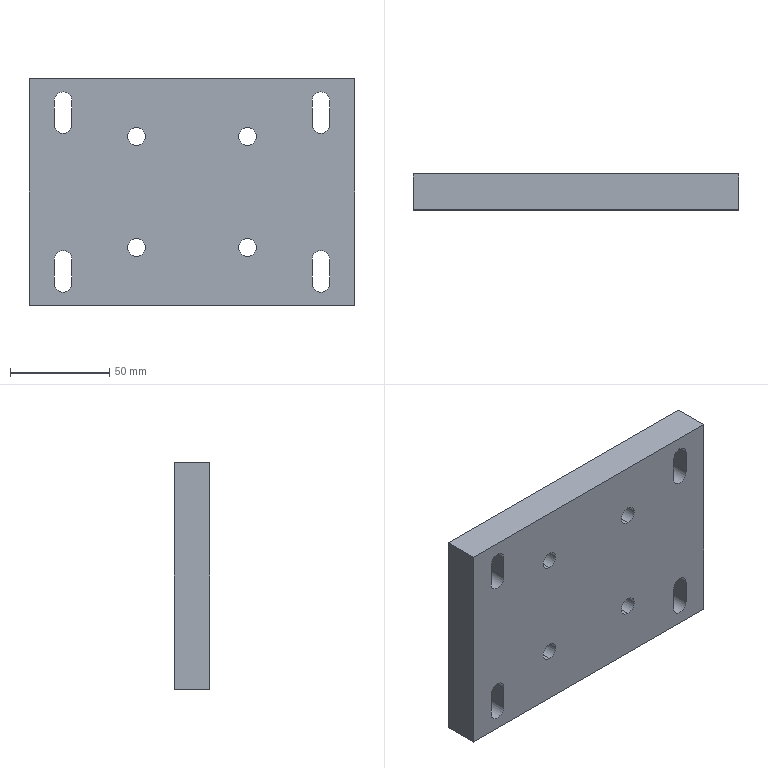Part | STEP file | PN_0058 (fixed plate) | 1 solid | 46 faces | box 164 x 18 x 114 mm | volume 315701 mm3 | cylinder 28 | plane 18 | commonest cylinder face diameters 9 x20 15 x8